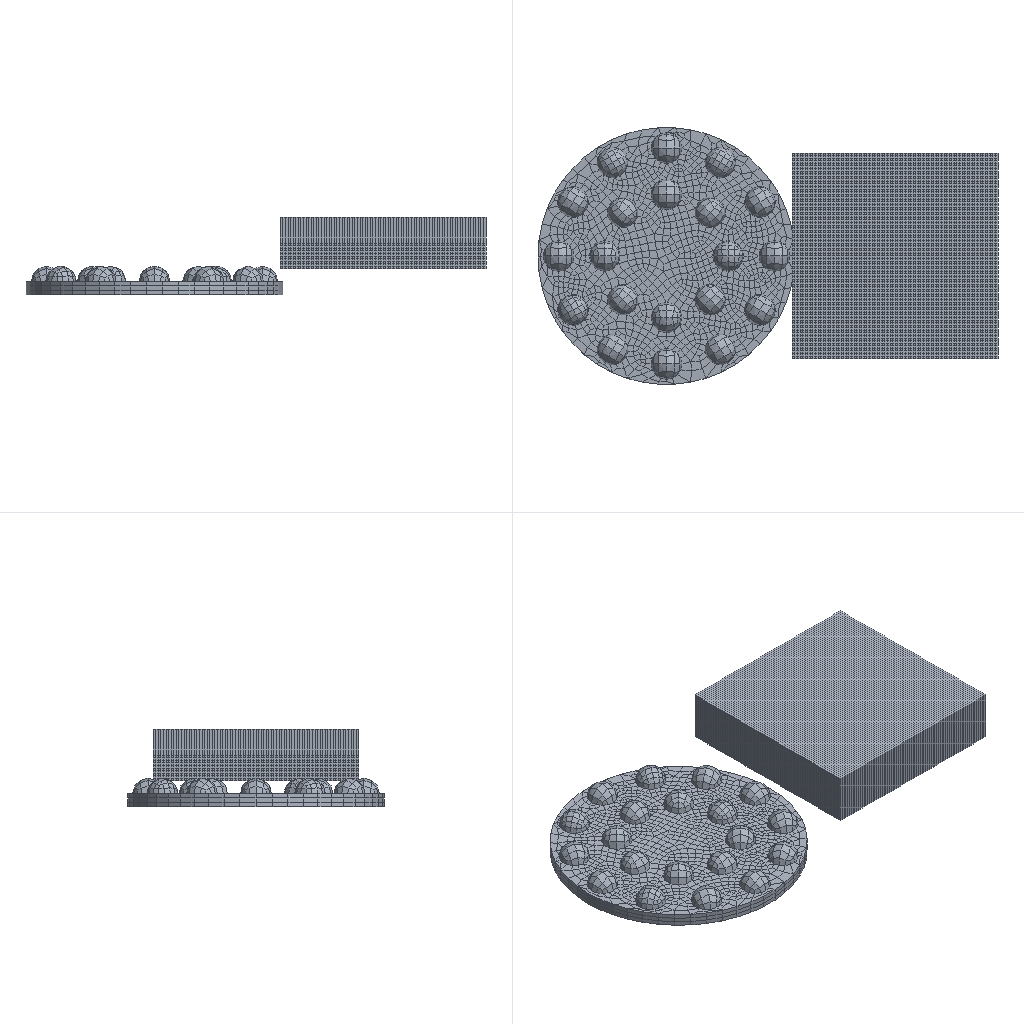Simulation study | abaqus
Set-up summary:
category,name,step,type,value,unit,region
solver,abaqus,,Abaqus/CAE 2024
units,SI m-kg-s (Pa),,inferred,E=1.68e+11 density=4492
analysis,Step-1,,dynamic explicit,nlgeom=True; time_period=6
mesh,nodes,,,87618
mesh,elements,,,77379
element_type,C3D8R,,,77379
material,daoju,,E,1.68e+11
material,daoju,,nu,0.23
material,daoju,,density,4492
material,daoju,,yield,1.2e+10
material,daoju,,conductivity,2000
material,daoju,,specific_heat,508
material,daoju,,behaviors,plastic; conductivity; damage initiation; damage evolution; specific heat
material,gongjian,,E,2e+11
material,gongjian,,nu,0.3
material,gongjian,,density,7850
material,gongjian,,yield,2.77e+08
material,gongjian,,behaviors,plastic; damage initiation; damage evolution; damage initiation; damage evolution; rate dependent
section,daoju,,solid section,,,_PickedSet65
section,gongjian,,solid section,,,_PickedSet9
bc,BC-1,initial,encastre,[dofs=ENCASTRE],,gongjian-1.gongjiandb
bc,BC-2,Step-1,velocity,"380 [dofs=rx,ry,rz,x,y,z n=6]",,daoju-1.rp
contact,Int-1,Step-1,contact pair,interaction=IntProp-1; friction=0.2; behavior=hard,,daoju-1.TOOLBIAOMIANA / gongjian-1_CHIP_CNS_
constraint,rigid body,,,1
Abaqus input file, long lists of numbers shortened:
*Heading
** Job name: deck Model name: Model-1
** Generated by: Abaqus/CAE 2024
*Preprint, echo=NO, model=NO, history=NO, contact=NO
**
** PARTS
**
*Part, name=daoju
*Node
      1,  0.6379, -0.6379,         0.25
      2,  0.85, -0.85,         0.25
** (8883 more lines like these left out)
*Element, type=C3D8R
 1,  897,  898, 4712, 4710,  124,  123,  887,  886
 2,  898,  129,  893, 4712,  123,    1,  128,  887
** (6977 more lines like these left out)
*Node
   8886,           0., 1.5308085e-16,           0.
*Nset, nset=daoju-RefPt_, internal
8886,
*Nset, nset=_PickedSet65, internal, generate
    1,  8885,     1
*Elset, elset=_PickedSet65, internal, generate
    1,  6979,     1
*Nset, nset=rp
 8886,
*Nset, nset=daojuti, generate
    1,  8886,     1
*Elset, elset=daojuti, generate
    1,  6979,     1
*Elset, elset=TOOLRIGID
 3394, 3395, 3396, 3397, 3398, 3399, 3400, 3401, 3402, 3403, 3404, 3405, 3406, 3407, 3408, 3409
 3410, 3411, 3412, 3413, 3414, 3415, 3416, 3417, 3418, 3419, 3420, 3421, 3422, 3423, 3424, 3425
** (190 more lines like these left out)
*Elset, elset=RIGIDA
 5187, 5188, 5189, 5190, 5191, 5192, 5193, 5194, 5195, 5196, 5197, 5198, 5199, 5200, 5201, 5202
 5203, 5204, 5205, 5206, 5207, 5208, 5209, 5210, 5211, 5212, 5213, 5214, 5215, 5216, 5217, 5218
** (78 more lines like these left out)
*Elset, elset=_daojumian_S2, internal
   41,   42,   45,   46,   47,   48,   53,   54,   61,   62,   65,   66,   69,   70,   71,   72
  101,  102,  105,  106,  109,  110,  111,  112,  161,  162,  165,  166,  167,  168,  173,  174
** (127 more lines like these left out)
*Elset, elset=_daojumian_S4, internal
    2,    4,   14,   16,   18,   20,   22,   24,   26,   28,   38,   40,   82,   84,   98,  100
  122,  124,  134,  136,  138,  140,  142,  144,  146,  148,  158,  160,  202,  204,  218,  220
** (20 more lines like these left out)
*Elset, elset=_daojumian_S3, internal
    9,   10,   33,   35,   89,   90,   93,   94,  129,  130,  153,  155,  209,  210,  213,  214
  269,  270,  273,  274,  333,  334,  335,  336,  389,  390,  393,  394,  425,  427,  437,  438
** (9 more lines like these left out)
*Elset, elset=_daojumian_S6, internal
 2420, 2487, 2525, 2549, 2550, 2569, 2592, 2602, 2663, 3112, 3293, 4213, 4280, 4318, 4342, 4343
 4362, 4385, 4395, 4456, 4905, 5086, 6006, 6073, 6111, 6135, 6136, 6155, 6178, 6188, 6249, 6698
** (1 more lines like these left out)
*Elset, elset=_daojumian_S5, internal
 2482, 2489, 2595, 2653, 2804, 2887, 2891, 2917, 2918, 3096, 3111, 3298, 3315, 3331, 3369, 4275
 4282, 4388, 4446, 4597, 4680, 4684, 4710, 4711, 4889, 4904, 5091, 5108, 5124, 5162, 6068, 6075
** (1 more lines like these left out)
*Elset, elset=_daojumian_S1, internal, generate
 5979,  6955,     1
*Surface, type=ELEMENT, name=daojumian
_daojumian_S2, S2
_daojumian_S4, S4
_daojumian_S6, S6
_daojumian_S3, S3
_daojumian_S5, S5
_daojumian_S1, S1
*Elset, elset=_TOOL-SURF_S1, internal, generate
 5979,  6955,     1
*Elset, elset=_TOOL-SURF_S2, internal
   41,   42,   45,   46,   47,   48,   53,   54,   61,   62,   65,   66,   69,   70,   71,   72
  101,  102,  105,  106,  109,  110,  111,  112,  161,  162,  165,  166,  167,  168,  173,  174
** (127 more lines like these left out)
*Elset, elset=_TOOL-SURF_S3, internal
    9,   10,   33,   35,   89,   90,   93,   94,  129,  130,  153,  155,  209,  210,  213,  214
  269,  270,  273,  274,  333,  334,  335,  336,  389,  390,  393,  394,  425,  427,  437,  438
** (9 more lines like these left out)
*Elset, elset=_TOOL-SURF_S4, internal
    2,    4,   14,   16,   18,   20,   22,   24,   26,   28,   38,   40,   82,   84,   98,  100
  122,  124,  134,  136,  138,  140,  142,  144,  146,  148,  158,  160,  202,  204,  218,  220
** (20 more lines like these left out)
*Elset, elset=_TOOL-SURF_S5, internal
 2482, 2489, 2595, 2653, 2804, 2887, 2891, 2917, 2918, 3096, 3111, 3298, 3315, 3331, 3369, 4275
 4282, 4388, 4446, 4597, 4680, 4684, 4710, 4711, 4889, 4904, 5091, 5108, 5124, 5162, 6068, 6075
** (1 more lines like these left out)
*Elset, elset=_TOOL-SURF_S6, internal
 2420, 2487, 2525, 2549, 2550, 2569, 2592, 2602, 2663, 3112, 3293, 4213, 4280, 4318, 4342, 4343
 4362, 4385, 4395, 4456, 4905, 5086, 6006, 6073, 6111, 6135, 6136, 6155, 6178, 6188, 6249, 6698
** (1 more lines like these left out)
*Surface, type=ELEMENT, name=TOOL-SURF
_TOOL-SURF_S1, S1
_TOOL-SURF_S2, S2
_TOOL-SURF_S4, S4
_TOOL-SURF_S6, S6
_TOOL-SURF_S3, S3
_TOOL-SURF_S5, S5
*Elset, elset=_TOOLBIAOMIAN_S2, internal
   41,   42,   45,   46,   47,   48,   53,   54,   61,   62,   65,   66,   69,   70,   71,   72
  101,  102,  105,  106,  109,  110,  111,  112,  161,  162,  165,  166,  167,  168,  173,  174
** (14 more lines like these left out)
*Elset, elset=_TOOLBIAOMIAN_S3, internal
    9,   10,   33,   35,   89,   90,   93,   94,  129,  130,  153,  155,  209,  210,  213,  214
  269,  270,  273,  274,  333,  334,  335,  389,  390,  393,  394,  425,  427,  437,  438,  445
** (7 more lines like these left out)
*Elset, elset=_TOOLBIAOMIAN_S4, internal
    2,    4,   14,   16,   18,   20,   22,   24,   26,   28,   38,   40,   82,   84,   98,  100
  122,  124,  134,  136,  138,  140,  142,  144,  146,  148,  158,  160,  202,  204,  218,  220
** (16 more lines like these left out)
*Surface, type=ELEMENT, name=TOOLBIAOMIAN
_TOOLBIAOMIAN_S2, S2
_TOOLBIAOMIAN_S3, S3
_TOOLBIAOMIAN_S4, S4
*Elset, elset=_TOOLBIAOMIANA_S2, internal
   41,   42,   45,   46,   47,   48,   53,   54,   61,   62,   65,   66,   69,   70,   71,   72
  101,  102,  105,  106,  109,  110,  111,  112,  161,  162,  165,  166,  167,  168,  173,  174
** (76 more lines like these left out)
*Elset, elset=_TOOLBIAOMIANA_S3, internal
    9,   10,   33,   35,   89,   90,   93,   94,  129,  130,  153,  155,  209,  210,  213,  214
  269,  270,  273,  274,  333,  334,  335,  336,  389,  390,  393,  394,  425,  427,  437,  438
** (8 more lines like these left out)
*Elset, elset=_TOOLBIAOMIANA_S4, internal
    2,    4,   14,   16,   18,   20,   22,   24,   26,   28,   38,   40,   82,   84,   98,  100
  122,  124,  134,  136,  138,  140,  142,  144,  146,  148,  158,  160,  202,  204,  218,  220
** (18 more lines like these left out)
*Elset, elset=_TOOLBIAOMIANA_S5, internal
 2482, 2489, 2595, 2653, 2804, 2887, 2891, 2917, 2918, 3096, 3111, 3298, 3315, 3331, 3369
*Elset, elset=_TOOLBIAOMIANA_S6, internal
 2420, 2487, 2525, 2549, 2550, 2569, 2592, 2602, 2663, 3112, 3293
*Surface, type=ELEMENT, name=TOOLBIAOMIANA
_TOOLBIAOMIANA_S2, S2
_TOOLBIAOMIANA_S3, S3
_TOOLBIAOMIANA_S4, S4
_TOOLBIAOMIANA_S6, S6
_TOOLBIAOMIANA_S5, S5
** Section: daoju
*Solid Section, elset=_PickedSet65, material=daoju
1.,
*End Part
**
*Part, name=gongjian
*Node
      1,          -2.,          -2.,          0.5
      2,          -2.,           2.,          0.5
** (78730 more lines like these left out)
*Element, type=C3D8R
    1,   522,  3841, 22564,  2419,     1,    13,   997,   188
    2,  3841,  3842, 22565, 22564,    13,    14,   998,   997
** (70398 more lines like these left out)
*Nset, nset=_PickedSet9, internal, generate
     1,  78732,      1
*Elset, elset=_PickedSet9, internal, generate
     1,  70400,      1
*Nset, nset=gongjiandb
     9,    10,    11,    12,   681,   682,   683,   684,   685,   686,   687,   688,   689,   690,   691,   692
   693,   694,   695,   696,   697,   698,   699,   700,   701,   702,   703,   704,   705,   706,   707,   708
** (409 more lines like these left out)
*Elset, elset=gongjiandb, generate
 64001,  70400,      1
*Nset, nset=CHIP
     3,     4,     6,     7,    92,    93,    94,    95,    96,    97,    98,    99,   100,   101,   102,   103
   104,   105,   106,   107,   108,   109,   110,   111,   112,   113,   114,   115,   116,   117,   118,   119
** (3886 more lines like these left out)
** Section: gongjian
*Solid Section, elset=_PickedSet9, controls=EC-1, material=gongjian
1.,
*End Part
**
**
** ASSEMBLY
**
*Assembly, name=Assembly
**
*Instance, name=daoju-1, part=daoju
*End Instance
**
*Instance, name=gongjian-1, part=gongjian
        4.45,           0.,          0.5
*End Instance
**
*Nset, nset=_PickedSet7, internal, instance=daoju-1
 8886,
*Surface, type=NODE, name=gongjian-1_CHIP_CNS_, internal
gongjian-1.CHIP, 1.
** Constraint: Constraint-1
*Rigid Body, ref node=_PickedSet7, elset=daoju-1.RIGIDA
*End Assembly
**
** ELEMENT CONTROLS
**
*Section Controls, name=EC-1, ELEMENT DELETION=YES, hourglass=ENHANCED
1., 1., 1.
**
** MATERIALS
**
*Material, name=daoju
*Conductivity
2000.,
*Damage Initiation, criterion=JOHNSON COOK
0.,  0.01, -1.66,    0.,    0., 3550.,   20.,    1.
*Damage Evolution, type=DISPLACEMENT
 0.0001,
*Density
4492.,
*Elastic
 1.68e+11, 0.23
*Plastic
 1.2e+10,0.
*Specific Heat
508.,
*Material, name=gongjian
*Damage Initiation, criterion=JOHNSON COOK
 0.1,  0.76,  1.57, 0.005, -0.84, 1723.,  298.,    1.
*Damage Evolution, type=DISPLACEMENT
 1.5,
*Damage Initiation, criterion=SHEAR
 0.95,0.,0.
*Damage Evolution, type=DISPLACEMENT
 0.1,
*Density
7850.,
*Elastic
 2e+11, 0.3
*Plastic, hardening=JOHNSON COOK
 2.77e+08, 5.56e+08,    0.794,    0.944,    1723.,     298.
*Rate Dependent, type=JOHNSON COOK
 0.0096,1.
**
** INTERACTION PROPERTIES
**
*Surface Interaction, name=IntProp-1
*Friction
 0.2,
*Surface Behavior, pressure-overclosure=HARD
**
** BOUNDARY CONDITIONS
**
** Name: BC-1 Type: Symmetry/Antisymmetry/Encastre
*Boundary
gongjian-1.gongjiandb, ENCASTRE
** ----------------------------------------------------------------
**
** STEP: Step-1
**
*Step, name=Step-1, nlgeom=YES
*Dynamic, Explicit
, 6.
*Bulk Viscosity
0.06, 1.2
** Mass Scaling: Semi-Automatic
**               Whole Model
*Fixed Mass Scaling, factor=200.
**
** BOUNDARY CONDITIONS
**
** Name: BC-2 Type: Velocity/Angular velocity
*Boundary, type=VELOCITY
daoju-1.rp, 1, 1, 3.
daoju-1.rp, 2, 2
daoju-1.rp, 3, 3
daoju-1.rp, 4, 4
daoju-1.rp, 5, 5
daoju-1.rp, 6, 6, 380.
**
** INTERACTIONS
**
** Interaction: Int-1
*Contact Pair, interaction=IntProp-1, mechanical constraint=KINEMATIC, cpset=Int-1
daoju-1.TOOLBIAOMIANA, gongjian-1_CHIP_CNS_
**
** OUTPUT REQUESTS
**
*Restart, write, number interval=1, time marks=NO
**
** FIELD OUTPUT: F-Output-1
**
*Output, field
*Node Output
A, RF, U, V
*Element Output, directions=YES
EVF, LE, PE, PEEQ, PEEQVAVG, PEVAVG, S, STATUS, SVAVG
*Contact Output
CSTRESS,
**
** HISTORY OUTPUT: H-Output-1
**
*Output, history, variable=PRESELECT
*End Step
Results summary:
result,odb.job_status,,,JOB_STATUS_COMPLETED_SUCCESSFULLY,"consistent, unstated (Abaqus has no unit system)"
result,steps[0].procedure,Step-1,,"*DYNAMIC, EXPLICIT","consistent, unstated (Abaqus has no unit system)"
result,steps[0].time_period,Step-1,,6,"consistent, unstated (Abaqus has no unit system)"
result,steps[0].n_frames,Step-1,,21,"consistent, unstated (Abaqus has no unit system)"
result,steps[0].last_frame.id,Step-1,,69132,"consistent, unstated (Abaqus has no unit system)"
result,steps[0].last_frame.value,Step-1,,6,"consistent, unstated (Abaqus has no unit system)"
result,steps[0].last_frame.description,Step-1,,Increment     69132: Step Time =    6.000,"consistent, unstated (Abaqus has no unit system)"
result,steps[0].completed,Step-1,,True,"consistent, unstated (Abaqus has no unit system)"
result,steps[0].max_U_magnitude,Step-1,,4122.15,"consistent, unstated (Abaqus has no unit system)"
result,steps[0].max_S_mises,Step-1,,1.25759e+09,"consistent, unstated (Abaqus has no unit system)"
result,steps[0].RF_sum[1],Step-1,,-9.38816e+10,"consistent, unstated (Abaqus has no unit system)"
result,steps[0].RF_sum[2],Step-1,,-9.36279e+10,"consistent, unstated (Abaqus has no unit system)"
result,steps[0].RF_sum[3],Step-1,,0,"consistent, unstated (Abaqus has no unit system)"
result,steps[0].diagnostic.n_increments,Step-1,,41,"consistent, unstated (Abaqus has no unit system)"